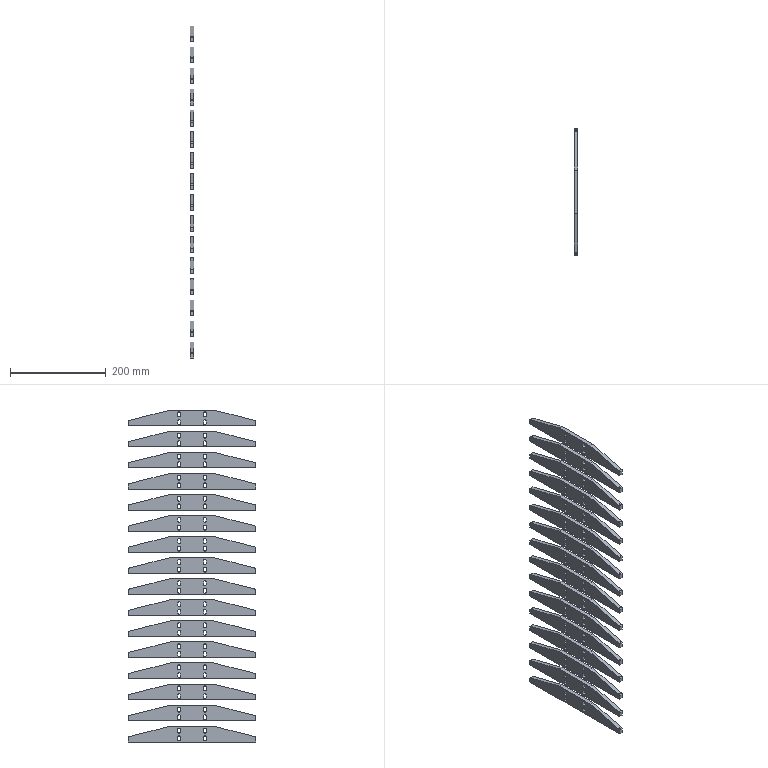Part | 16 solids | 576 faces | box 8 x 265.5 x 693 mm | volume 840174 mm3 | plane 336 | cylinder 240 | commonest cylinder face diameters 5.5 x128 3.2 x80 6 x32